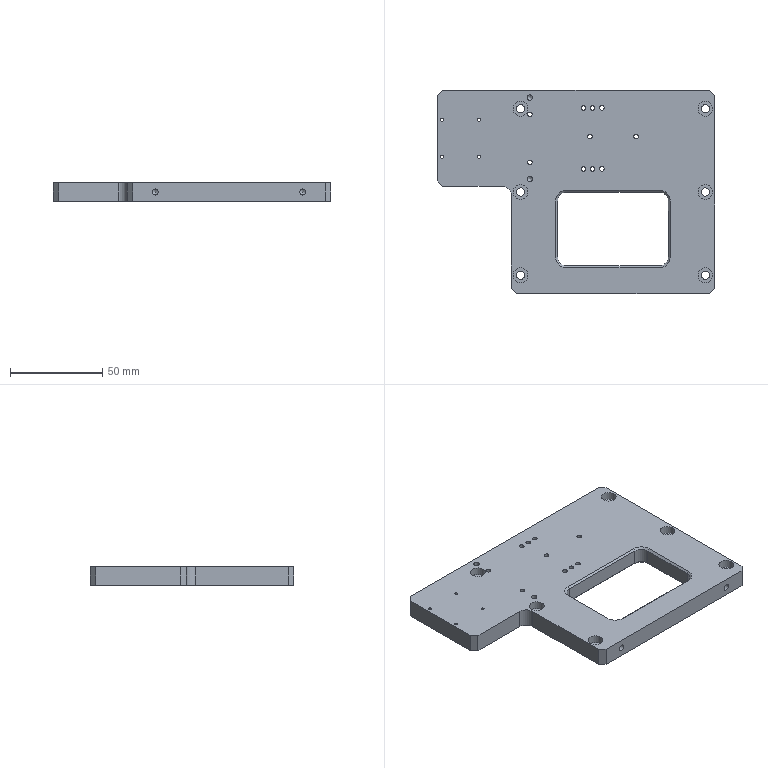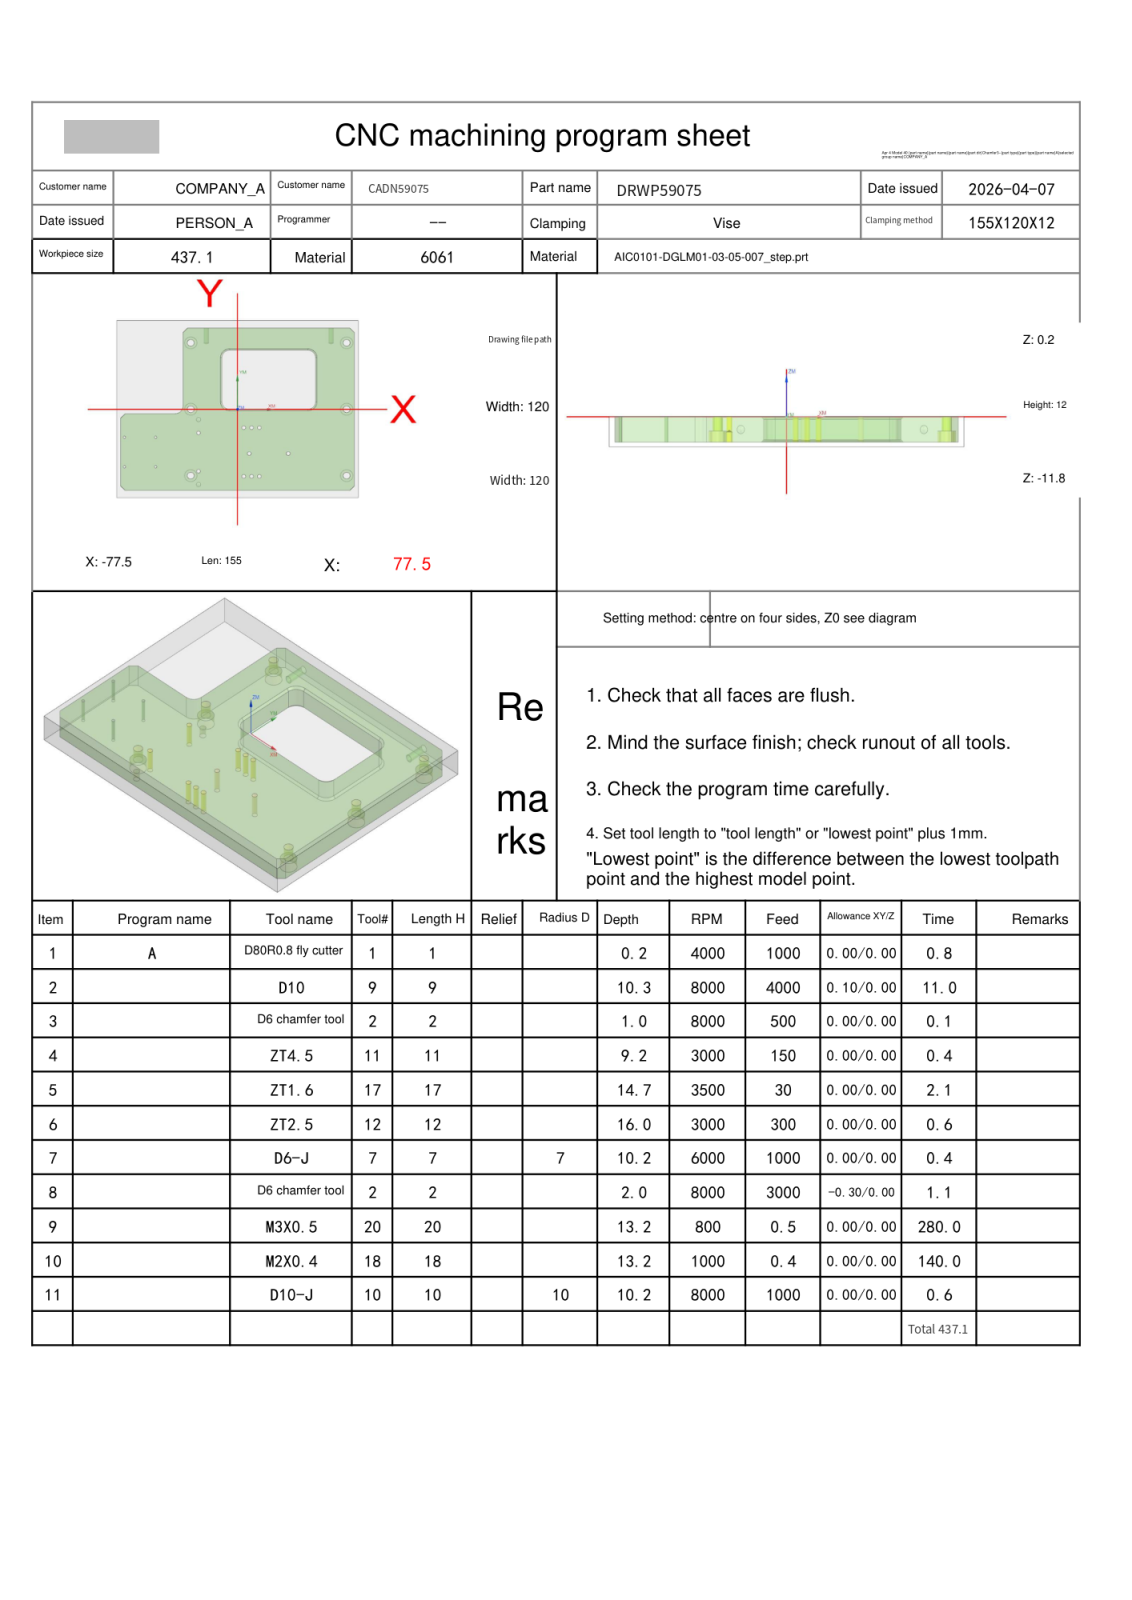NC program | NX | posted by the shop | part box 150 x 110 x 10 mm
Lines 41 to 1212 of 3675:
N2 T09 M06
(D10  D=10. R=0. H=09 ce=0.10 di=0.10)
G00 G90 G54 X-89.5 Y21.5 M03 S8000
G43 H09 Z10.2
M08
Z.719
G01 Z-.481 F4000.
X-85.
G03 X-78. Y28.5 I0.0 J7.
G01 Y60.
G02 X-77.5 Y60.5 I.5 J0.0
G01 X-35.464
G02 X-32. Y61.5 I3.464 J-5.5
G01 X72.
G02 X75.464 Y60.5 I0.0 J-6.5
G01 X77.5
G02 X78. Y60. I0.0 J-.5
G01 Y58.192
X79.596 Y56.596
G02 X81.5 Y52. I-4.596 J-4.596
G01 Y-52.
G02 X79.596 Y-56.596 I-6.5 J0.0
G01 X78. Y-58.192
Y-60.
G02 X77.5 Y-60.5 I-.5 J0.0
G01 X75.464
G02 X72. Y-61.5 I-3.464 J5.5
G01 X-72.
G02 X-75.464 Y-60.5 I0.0 J6.5
G01 X-77.5
G02 X-78. Y-60. I0.0 J.5
G01 Y-58.192
X-79.596 Y-56.596
G02 X-81.5 Y-52. I4.596 J4.596
G01 Y-6.
G02 X-79.596 Y-1.404 I6.5 J0.0
G01 X-78. Y.192
Y30.486
G02 X-77.582 Y31.299 I1. J0.0
G01 X-71.418 Y35.701
G03 X-71. Y36.514 I-.582 J.814
G01 Y52.503
G02 X-70.003 Y53.5 I1. J-.003
G01 X-42.48
G02 X-41.483 Y52.5 I-.003 J-1.
G01 X-41.485 Y52.436
G03 X-41.5 Y52. I6.485 J-.436
G01 Y4.497
G02 X-42.497 Y3.5 I-1. J.003
G01 X-69.511
G03 X-70.214 Y3.055 I0.0 J-.779
G01 X-70.383 Y2.7
X-70.423 Y2.52
G03 X-70.003 Y2.1 I.42 J0.0
G01 X-40.1
Y52.
G02 X-38.606 Y55.606 I5.1 J0.0
G01 X-35.606 Y58.606
G02 X-32. Y60.1 I3.606 J-3.606
G01 X72.
G02 X75.606 Y58.606 I0.0 J-5.1
G01 X78.606 Y55.606
G02 X80.1 Y52. I-3.606 J-3.606
G01 Y-52.
G02 X78.606 Y-55.606 I-5.1 J0.0
G01 X75.606 Y-58.606
G02 X72. Y-60.1 I-3.606 J3.606
G01 X-72.
G02 X-75.606 Y-58.606 I0.0 J5.1
G01 X-78.606 Y-55.606
G02 X-80.1 Y-52. I3.606 J3.606
G01 Y-6.
G02 X-78.606 Y-2.394 I5.1 J0.0
G01 X-75.606 Y.606
G02 X-72. Y2.1 I3.606 J-3.606
G01 X-70.003
G03 X-69.583 Y2.52 I0.0 J.42
G01 X-69.624 Y2.7
X-69.907 Y3.298
G03 X-70.191 Y3.518 I-.361 J-.172
G02 X-71. Y4.497 I.191 J.981
G01 Y30.486
G02 X-70.582 Y31.299 I1. J0.0
G01 X-64.418 Y35.701
G03 X-64. Y36.514 I-.582 J.814
G01 Y45.503
G02 X-63.003 Y46.5 I1. J-.003
G01 X-49.497
G02 X-48.5 Y45.503 I-.003 J-1.
G01 Y11.497
G02 X-49.497 Y10.5 I-1. J.003
G01 X-63.003
G02 X-64. Y11.497 I.003 J1.
G01 Y30.486
G02 X-63.582 Y31.299 I1. J0.0
G01 X-57.419 Y35.701
G03 X-57. Y36.514 I-.581 J.814
G01 Y38.803
G02 X-56.303 Y39.5 I.7 J-.003
G01 X-56.197
G02 X-55.5 Y38.803 I-.003 J-.7
G01 Y18.197
G02 X-56.197 Y17.5 I-.7 J.003
G01 X-56.303
G02 X-57. Y18.197 I.003 J.7
G01 Y33.5
Y34.
G03 X-64. Y41. I-7. J0.0
G01 X-89.5
Z.719
G00 Z3.
G01 Y21.5 F6000.
G00 Z.238
G01 Z-.962 F4000.
X-85.
G03 X-78. Y28.5 I0.0 J7.
G01 Y60.
G02 X-77.5 Y60.5 I.5 J0.0
G01 X-35.464
G02 X-32. Y61.5 I3.464 J-5.5
G01 X72.
G02 X75.464 Y60.5 I0.0 J-6.5
G01 X77.5
G02 X78. Y60. I0.0 J-.5
G01 Y58.192
X79.596 Y56.596
G02 X81.5 Y52. I-4.596 J-4.596
G01 Y-52.
G02 X79.596 Y-56.596 I-6.5 J0.0
G01 X78. Y-58.192
Y-60.
G02 X77.5 Y-60.5 I-.5 J0.0
G01 X75.464
G02 X72. Y-61.5 I-3.464 J5.5
G01 X-72.
G02 X-75.464 Y-60.5 I0.0 J6.5
G01 X-77.5
G02 X-78. Y-60. I0.0 J.5
G01 Y-58.192
X-79.596 Y-56.596
G02 X-81.5 Y-52. I4.596 J4.596
G01 Y-6.
G02 X-79.596 Y-1.404 I6.5 J0.0
G01 X-78. Y.192
Y33.5
G02 X-77.238 Y34.471 I1. J0.0
G01 X-71.762 Y35.813
G03 X-71. Y36.784 I-.238 J.971
G01 Y52.503
G02 X-70.003 Y53.5 I1. J-.003
G01 X-42.481
G02 X-41.483 Y52.5 I-.003 J-1.
G01 X-41.485 Y52.436
G03 X-41.5 Y52. I6.485 J-.436
G01 Y4.497
G02 X-42.497 Y3.5 I-1. J.003
G01 X-69.51
G03 X-70.214 Y3.055 I0.0 J-.779
G01 X-70.382 Y2.7
X-70.423 Y2.52
G03 X-70.003 Y2.1 I.42 J0.0
G01 X-40.1
Y52.
G02 X-38.606 Y55.606 I5.1 J0.0
G01 X-35.606 Y58.606
G02 X-32. Y60.1 I3.606 J-3.606
G01 X72.
G02 X75.606 Y58.606 I0.0 J-5.1
G01 X78.606 Y55.606
G02 X80.1 Y52. I-3.606 J-3.606
G01 Y-52.
G02 X78.606 Y-55.606 I-5.1 J0.0
G01 X75.606 Y-58.606
G02 X72. Y-60.1 I-3.606 J3.606
G01 X-72.
G02 X-75.606 Y-58.606 I0.0 J5.1
G01 X-78.606 Y-55.606
G02 X-80.1 Y-52. I3.606 J3.606
G01 Y-6.
G02 X-78.606 Y-2.394 I5.1 J0.0
G01 X-75.606 Y.606
G02 X-72. Y2.1 I3.606 J-3.606
G01 X-70.003
G03 X-69.583 Y2.52 I0.0 J.42
G01 X-69.623 Y2.7
X-69.906 Y3.298
G03 X-70.191 Y3.518 I-.361 J-.172
G02 X-71. Y4.497 I.191 J.982
G01 Y30.486
G02 X-70.582 Y31.299 I1. J0.0
G01 X-64.418 Y35.701
G03 X-64. Y36.514 I-.582 J.814
G01 Y45.503
G02 X-63.003 Y46.5 I1. J-.003
G01 X-49.497
G02 X-48.5 Y45.503 I-.003 J-1.
G01 Y11.497
G02 X-49.497 Y10.5 I-1. J.003
G01 X-63.003
G02 X-64. Y11.497 I.003 J1.
G01 Y30.486
G02 X-63.582 Y31.299 I1. J0.0
G01 X-57.419 Y35.701
G03 X-57. Y36.514 I-.581 J.814
G01 Y38.803
G02 X-56.303 Y39.5 I.7 J-.003
G01 X-56.197
G02 X-55.5 Y38.803 I-.003 J-.7
G01 Y18.197
G02 X-56.197 Y17.5 I-.7 J.003
G01 X-56.303
G02 X-57. Y18.197 I.003 J.7
G01 Y33.5
Y34.
G03 X-64. Y41. I-7. J0.0
G01 X-89.5
Z.238
G00 Z2.519
G01 Y21.5 F6000.
G00 Z-.243
G01 Z-1.443 F4000.
X-85.
G03 X-78. Y28.5 I0.0 J7.
G01 Y60.
G02 X-77.5 Y60.5 I.5 J0.0
G01 X-35.464
G02 X-32. Y61.5 I3.464 J-5.5
G01 X72.
G02 X75.464 Y60.5 I0.0 J-6.5
G01 X77.5
G02 X78. Y60. I0.0 J-.5
G01 Y58.192
X79.596 Y56.596
G02 X81.5 Y52. I-4.596 J-4.596
G01 Y-52.
G02 X79.596 Y-56.596 I-6.5 J0.0
G01 X78. Y-58.192
Y-60.
G02 X77.5 Y-60.5 I-.5 J0.0
G01 X75.464
G02 X72. Y-61.5 I-3.464 J5.5
G01 X-72.
G02 X-75.464 Y-60.5 I0.0 J6.5
G01 X-77.5
G02 X-78. Y-60. I0.0 J.5
G01 Y-58.192
X-79.596 Y-56.596
G02 X-81.5 Y-52. I4.596 J4.596
G01 Y-6.
G02 X-79.596 Y-1.404 I6.5 J0.0
G01 X-78. Y.192
Y33.5
G02 X-77.238 Y34.471 I1. J0.0
G01 X-71.762 Y35.813
G03 X-71. Y36.784 I-.238 J.971
G01 Y52.503
G02 X-70.003 Y53.5 I1. J-.003
G01 X-42.481
G02 X-41.483 Y52.5 I-.003 J-1.
G01 X-41.485 Y52.436
G03 X-41.5 Y52. I6.485 J-.436
G01 Y4.497
G02 X-42.497 Y3.5 I-1. J.003
G01 X-69.51
G03 X-70.214 Y3.055 I0.0 J-.779
G01 X-70.382 Y2.7
X-70.423 Y2.52
G03 X-70.003 Y2.1 I.42 J0.0
G01 X-40.1
Y52.
G02 X-38.606 Y55.606 I5.1 J0.0
G01 X-35.606 Y58.606
G02 X-32. Y60.1 I3.606 J-3.606
G01 X72.
G02 X75.606 Y58.606 I0.0 J-5.1
G01 X78.606 Y55.606
G02 X80.1 Y52. I-3.606 J-3.606
G01 Y-52.
G02 X78.606 Y-55.606 I-5.1 J0.0
G01 X75.606 Y-58.606
G02 X72. Y-60.1 I-3.606 J3.606
G01 X-72.
G02 X-75.606 Y-58.606 I0.0 J5.1
G01 X-78.606 Y-55.606
G02 X-80.1 Y-52. I3.606 J3.606
G01 Y-6.
G02 X-78.606 Y-2.394 I5.1 J0.0
G01 X-75.606 Y.606
G02 X-72. Y2.1 I3.606 J-3.606
G01 X-70.003
G03 X-69.583 Y2.52 I0.0 J.42
G01 X-69.623 Y2.7
X-69.906 Y3.298
G03 X-70.191 Y3.518 I-.361 J-.172
G02 X-71. Y4.497 I.191 J.982
G01 Y30.486
G02 X-70.582 Y31.299 I1. J0.0
G01 X-64.418 Y35.701
G03 X-64. Y36.514 I-.582 J.814
G01 Y45.503
G02 X-63.003 Y46.5 I1. J-.003
G01 X-49.497
G02 X-48.5 Y45.503 I-.003 J-1.
G01 Y11.497
G02 X-49.497 Y10.5 I-1. J.003
G01 X-63.003
G02 X-64. Y11.497 I.003 J1.
G01 Y30.486
G02 X-63.582 Y31.299 I1. J0.0
G01 X-57.419 Y35.701
G03 X-57. Y36.514 I-.581 J.814
G01 Y38.803
G02 X-56.303 Y39.5 I.7 J-.003
G01 X-56.197
G02 X-55.5 Y38.803 I-.003 J-.7
G01 Y18.197
G02 X-56.197 Y17.5 I-.7 J.003
G01 X-56.303
G02 X-57. Y18.197 I.003 J.7
G01 Y33.5
Y34.
G03 X-64. Y41. I-7. J0.0
G01 X-89.5
Z-.243
G00 Z2.038
G01 Y21.5 F6000.
G00 Z-.724
G01 Z-1.924 F4000.
X-85.
G03 X-78. Y28.5 I0.0 J7.
G01 Y60.
G02 X-77.5 Y60.5 I.5 J0.0
G01 X-35.464
G02 X-32. Y61.5 I3.464 J-5.5
G01 X72.
G02 X75.464 Y60.5 I0.0 J-6.5
G01 X77.5
G02 X78. Y60. I0.0 J-.5
G01 Y58.192
X79.596 Y56.596
G02 X81.5 Y52. I-4.596 J-4.596
G01 Y-52.
G02 X79.596 Y-56.596 I-6.5 J0.0
G01 X78. Y-58.192
Y-60.
G02 X77.5 Y-60.5 I-.5 J0.0
G01 X75.464
G02 X72. Y-61.5 I-3.464 J5.5
G01 X-72.
G02 X-75.464 Y-60.5 I0.0 J6.5
G01 X-77.5
G02 X-78. Y-60. I0.0 J.5
G01 Y-58.192
X-79.596 Y-56.596
G02 X-81.5 Y-52. I4.596 J4.596
G01 Y-6.
G02 X-79.596 Y-1.404 I6.5 J0.0
G01 X-78. Y.192
Y33.5
G02 X-77.238 Y34.471 I1. J0.0
G01 X-71.762 Y35.813
G03 X-71. Y36.784 I-.238 J.971
G01 Y52.503
G02 X-70.003 Y53.5 I1. J-.003
G01 X-42.481
G02 X-41.483 Y52.5 I-.003 J-1.
G01 X-41.485 Y52.436
G03 X-41.5 Y52. I6.485 J-.436
G01 Y4.497
G02 X-42.497 Y3.5 I-1. J.003
G01 X-69.51
G03 X-70.214 Y3.055 I0.0 J-.779
G01 X-70.382 Y2.7
X-70.423 Y2.52
G03 X-70.003 Y2.1 I.42 J0.0
G01 X-40.1
Y52.
G02 X-38.606 Y55.606 I5.1 J0.0
G01 X-35.606 Y58.606
G02 X-32. Y60.1 I3.606 J-3.606
G01 X72.
G02 X75.606 Y58.606 I0.0 J-5.1
G01 X78.606 Y55.606
G02 X80.1 Y52. I-3.606 J-3.606
G01 Y-52.
G02 X78.606 Y-55.606 I-5.1 J0.0
G01 X75.606 Y-58.606
G02 X72. Y-60.1 I-3.606 J3.606
G01 X-72.
G02 X-75.606 Y-58.606 I0.0 J5.1
G01 X-78.606 Y-55.606
G02 X-80.1 Y-52. I3.606 J3.606
G01 Y-6.
G02 X-78.606 Y-2.394 I5.1 J0.0
G01 X-75.606 Y.606
G02 X-72. Y2.1 I3.606 J-3.606
G01 X-70.003
G03 X-69.583 Y2.52 I0.0 J.42
G01 X-69.623 Y2.7
X-69.906 Y3.298
G03 X-70.191 Y3.518 I-.361 J-.172
G02 X-71. Y4.497 I.191 J.982
G01 Y30.486
G02 X-70.582 Y31.299 I1. J0.0
G01 X-64.418 Y35.701
G03 X-64. Y36.514 I-.582 J.814
G01 Y45.503
G02 X-63.003 Y46.5 I1. J-.003
G01 X-49.497
G02 X-48.5 Y45.503 I-.003 J-1.
G01 Y11.497
G02 X-49.497 Y10.5 I-1. J.003
G01 X-63.003
G02 X-64. Y11.497 I.003 J1.
G01 Y30.486
G02 X-63.582 Y31.299 I1. J0.0
G01 X-57.419 Y35.701
G03 X-57. Y36.514 I-.581 J.814
G01 Y38.803
G02 X-56.303 Y39.5 I.7 J-.003
G01 X-56.197
G02 X-55.5 Y38.803 I-.003 J-.7
G01 Y18.197
G02 X-56.197 Y17.5 I-.7 J.003
G01 X-56.303
G02 X-57. Y18.197 I.003 J.7
G01 Y33.5
Y34.
G03 X-64. Y41. I-7. J0.0
G01 X-89.5
Z-.724
G00 Z1.557
G01 Y21.5 F6000.
G00 Z-1.205
G01 Z-2.405 F4000.
X-85.
G03 X-78. Y28.5 I0.0 J7.
G01 Y60.
G02 X-77.5 Y60.5 I.5 J0.0
G01 X-35.464
G02 X-32. Y61.5 I3.464 J-5.5
G01 X72.
G02 X75.464 Y60.5 I0.0 J-6.5
G01 X77.5
G02 X78. Y60. I0.0 J-.5
G01 Y58.192
X79.596 Y56.596
G02 X81.5 Y52. I-4.596 J-4.596
G01 Y-52.
G02 X79.596 Y-56.596 I-6.5 J0.0
G01 X78. Y-58.192
Y-60.
G02 X77.5 Y-60.5 I-.5 J0.0
G01 X75.464
G02 X72. Y-61.5 I-3.464 J5.5
G01 X-72.
G02 X-75.464 Y-60.5 I0.0 J6.5
G01 X-77.5
G02 X-78. Y-60. I0.0 J.5
G01 Y-58.192
X-79.596 Y-56.596
G02 X-81.5 Y-52. I4.596 J4.596
G01 Y-6.
G02 X-79.596 Y-1.404 I6.5 J0.0
G01 X-78. Y.192
Y33.5
G02 X-77.238 Y34.471 I1. J0.0
G01 X-71.762 Y35.813
G03 X-71. Y36.784 I-.238 J.971
G01 Y52.503
G02 X-70.003 Y53.5 I1. J-.003
G01 X-42.481
G02 X-41.483 Y52.5 I-.003 J-1.
G01 X-41.485 Y52.436
G03 X-41.5 Y52. I6.485 J-.436
G01 Y4.497
G02 X-42.497 Y3.5 I-1. J.003
G01 X-69.51
G03 X-70.214 Y3.055 I0.0 J-.779
G01 X-70.382 Y2.7
X-70.423 Y2.52
G03 X-70.003 Y2.1 I.42 J0.0
G01 X-40.1
Y52.
G02 X-38.606 Y55.606 I5.1 J0.0
G01 X-35.606 Y58.606
G02 X-32. Y60.1 I3.606 J-3.606
G01 X72.
G02 X75.606 Y58.606 I0.0 J-5.1
G01 X78.606 Y55.606
G02 X80.1 Y52. I-3.606 J-3.606
G01 Y-52.
G02 X78.606 Y-55.606 I-5.1 J0.0
G01 X75.606 Y-58.606
G02 X72. Y-60.1 I-3.606 J3.606
G01 X-72.
G02 X-75.606 Y-58.606 I0.0 J5.1
G01 X-78.606 Y-55.606
G02 X-80.1 Y-52. I3.606 J3.606
G01 Y-6.
G02 X-78.606 Y-2.394 I5.1 J0.0
G01 X-75.606 Y.606
G02 X-72. Y2.1 I3.606 J-3.606
G01 X-70.003
G03 X-69.583 Y2.52 I0.0 J.42
G01 X-69.623 Y2.7
X-69.906 Y3.298
G03 X-70.191 Y3.518 I-.361 J-.172
G02 X-71. Y4.497 I.191 J.982
G01 Y30.486
G02 X-70.582 Y31.299 I1. J0.0
G01 X-64.418 Y35.701
G03 X-64. Y36.514 I-.582 J.814
G01 Y45.503
G02 X-63.003 Y46.5 I1. J-.003
G01 X-49.497
G02 X-48.5 Y45.503 I-.003 J-1.
G01 Y11.497
G02 X-49.497 Y10.5 I-1. J.003
G01 X-63.003
G02 X-64. Y11.497 I.003 J1.
G01 Y30.486
G02 X-63.582 Y31.299 I1. J0.0
G01 X-57.419 Y35.701
G03 X-57. Y36.514 I-.581 J.814
G01 Y38.803
G02 X-56.303 Y39.5 I.7 J-.003
G01 X-56.197
G02 X-55.5 Y38.803 I-.003 J-.7
G01 Y18.197
G02 X-56.197 Y17.5 I-.7 J.003
G01 X-56.303
G02 X-57. Y18.197 I.003 J.7
G01 Y33.5
Y34.
G03 X-64. Y41. I-7. J0.0
G01 X-89.5
Z-1.205
G00 Z1.076
G01 Y21.5 F6000.
G00 Z-1.686
G01 Z-2.886 F4000.
X-85.
G03 X-78. Y28.5 I0.0 J7.
G01 Y60.
G02 X-77.5 Y60.5 I.5 J0.0
G01 X-35.464
G02 X-32. Y61.5 I3.464 J-5.5
G01 X72.
G02 X75.464 Y60.5 I0.0 J-6.5
G01 X77.5
G02 X78. Y60. I0.0 J-.5
G01 Y58.192
X79.596 Y56.596
G02 X81.5 Y52. I-4.596 J-4.596
G01 Y-52.
G02 X79.596 Y-56.596 I-6.5 J0.0
G01 X78. Y-58.192
Y-60.
G02 X77.5 Y-60.5 I-.5 J0.0
G01 X75.464
G02 X72. Y-61.5 I-3.464 J5.5
G01 X-72.
G02 X-75.464 Y-60.5 I0.0 J6.5
G01 X-77.5
G02 X-78. Y-60. I0.0 J.5
G01 Y-58.192
X-79.596 Y-56.596
G02 X-81.5 Y-52. I4.596 J4.596
G01 Y-6.
G02 X-79.596 Y-1.404 I6.5 J0.0
G01 X-78. Y.192
Y33.5
G02 X-77.238 Y34.471 I1. J0.0
G01 X-71.762 Y35.813
G03 X-71. Y36.784 I-.238 J.971
G01 Y52.503
G02 X-70.003 Y53.5 I1. J-.003
G01 X-42.481
G02 X-41.483 Y52.5 I-.003 J-1.
G01 X-41.485 Y52.436
G03 X-41.5 Y52. I6.485 J-.436
G01 Y4.497
G02 X-42.497 Y3.5 I-1. J.003
G01 X-69.51
G03 X-70.214 Y3.055 I0.0 J-.779
G01 X-70.382 Y2.7
X-70.423 Y2.52
G03 X-70.003 Y2.1 I.42 J0.0
G01 X-40.1
Y52.
G02 X-38.606 Y55.606 I5.1 J0.0
G01 X-35.606 Y58.606
G02 X-32. Y60.1 I3.606 J-3.606
G01 X72.
G02 X75.606 Y58.606 I0.0 J-5.1
G01 X78.606 Y55.606
G02 X80.1 Y52. I-3.606 J-3.606
G01 Y-52.
G02 X78.606 Y-55.606 I-5.1 J0.0
G01 X75.606 Y-58.606
G02 X72. Y-60.1 I-3.606 J3.606
G01 X-72.
G02 X-75.606 Y-58.606 I0.0 J5.1
G01 X-78.606 Y-55.606
G02 X-80.1 Y-52. I3.606 J3.606
G01 Y-6.
G02 X-78.606 Y-2.394 I5.1 J0.0
G01 X-75.606 Y.606
G02 X-72. Y2.1 I3.606 J-3.606
G01 X-70.003
G03 X-69.583 Y2.52 I0.0 J.42
G01 X-69.623 Y2.7
X-69.906 Y3.298
G03 X-70.191 Y3.518 I-.361 J-.172
G02 X-71. Y4.497 I.191 J.982
G01 Y30.486
G02 X-70.582 Y31.299 I1. J0.0
G01 X-64.418 Y35.701
G03 X-64. Y36.514 I-.582 J.814
G01 Y45.503
G02 X-63.003 Y46.5 I1. J-.003
G01 X-49.497
G02 X-48.5 Y45.503 I-.003 J-1.
G01 Y11.497
G02 X-49.497 Y10.5 I-1. J.003
G01 X-63.003
G02 X-64. Y11.497 I.003 J1.
G01 Y30.486
G02 X-63.582 Y31.299 I1. J0.0
G01 X-57.419 Y35.701
G03 X-57. Y36.514 I-.581 J.814
G01 Y38.803
G02 X-56.303 Y39.5 I.7 J-.003
G01 X-56.197
G02 X-55.5 Y38.803 I-.003 J-.7
G01 Y18.197
G02 X-56.197 Y17.5 I-.7 J.003
G01 X-56.303
G02 X-57. Y18.197 I.003 J.7
G01 Y33.5
Y34.
G03 X-64. Y41. I-7. J0.0
G01 X-89.5
Z-1.686
G00 Z.595
G01 Y21.5 F6000.
G00 Z-2.167
G01 Z-3.367 F4000.
X-85.
G03 X-78. Y28.5 I0.0 J7.
G01 Y60.
G02 X-77.5 Y60.5 I.5 J0.0
G01 X-35.464
G02 X-32. Y61.5 I3.464 J-5.5
G01 X72.
G02 X75.464 Y60.5 I0.0 J-6.5
G01 X77.5
G02 X78. Y60. I0.0 J-.5
G01 Y58.192
X79.596 Y56.596
G02 X81.5 Y52. I-4.596 J-4.596
G01 Y-52.
G02 X79.596 Y-56.596 I-6.5 J0.0
G01 X78. Y-58.192
Y-60.
G02 X77.5 Y-60.5 I-.5 J0.0
G01 X75.464
G02 X72. Y-61.5 I-3.464 J5.5
G01 X-72.
G02 X-75.464 Y-60.5 I0.0 J6.5
G01 X-77.5
G02 X-78. Y-60. I0.0 J.5
G01 Y-58.192
X-79.596 Y-56.596
G02 X-81.5 Y-52. I4.596 J4.596
G01 Y-6.
G02 X-79.596 Y-1.404 I6.5 J0.0
G01 X-78. Y.192
Y33.5
G02 X-77.238 Y34.471 I1. J0.0
G01 X-71.762 Y35.813
G03 X-71. Y36.784 I-.238 J.971
G01 Y52.503
G02 X-70.003 Y53.5 I1. J-.003
G01 X-42.481
G02 X-41.483 Y52.5 I-.003 J-1.
G01 X-41.485 Y52.436
G03 X-41.5 Y52. I6.485 J-.436
G01 Y4.497
G02 X-42.497 Y3.5 I-1. J.003
G01 X-69.51
G03 X-70.214 Y3.055 I0.0 J-.779
G01 X-70.382 Y2.7
X-70.423 Y2.52
G03 X-70.003 Y2.1 I.42 J0.0
G01 X-40.1
Y52.
G02 X-38.606 Y55.606 I5.1 J0.0
G01 X-35.606 Y58.606
G02 X-32. Y60.1 I3.606 J-3.606
G01 X72.
G02 X75.606 Y58.606 I0.0 J-5.1
G01 X78.606 Y55.606
G02 X80.1 Y52. I-3.606 J-3.606
G01 Y-52.
G02 X78.606 Y-55.606 I-5.1 J0.0
G01 X75.606 Y-58.606
G02 X72. Y-60.1 I-3.606 J3.606
G01 X-72.
G02 X-75.606 Y-58.606 I0.0 J5.1
G01 X-78.606 Y-55.606
G02 X-80.1 Y-52. I3.606 J3.606
G01 Y-6.
G02 X-78.606 Y-2.394 I5.1 J0.0
G01 X-75.606 Y.606
G02 X-72. Y2.1 I3.606 J-3.606
G01 X-70.003
G03 X-69.583 Y2.52 I0.0 J.42
G01 X-69.623 Y2.7
X-69.906 Y3.298
G03 X-70.191 Y3.518 I-.361 J-.172
G02 X-71. Y4.497 I.191 J.982
G01 Y30.486
G02 X-70.582 Y31.299 I1. J0.0
G01 X-64.418 Y35.701
G03 X-64. Y36.514 I-.582 J.814
G01 Y45.503
G02 X-63.003 Y46.5 I1. J-.003
G01 X-49.497
G02 X-48.5 Y45.503 I-.003 J-1.
G01 Y11.497
G02 X-49.497 Y10.5 I-1. J.003
G01 X-63.003
G02 X-64. Y11.497 I.003 J1.
G01 Y30.486
G02 X-63.582 Y31.299 I1. J0.0
G01 X-57.419 Y35.701
G03 X-57. Y36.514 I-.581 J.814
G01 Y38.803
G02 X-56.303 Y39.5 I.7 J-.003
G01 X-56.197
G02 X-55.5 Y38.803 I-.003 J-.7
G01 Y18.197
G02 X-56.197 Y17.5 I-.7 J.003
G01 X-56.303
G02 X-57. Y18.197 I.003 J.7
G01 Y33.5
Y34.
G03 X-64. Y41. I-7. J0.0
G01 X-89.5
Z-2.167
G00 Z.114
G01 Y21.5 F6000.
G00 Z-2.648
G01 Z-3.848 F4000.
X-85.
G03 X-78. Y28.5 I0.0 J7.
G01 Y60.
G02 X-77.5 Y60.5 I.5 J0.0
G01 X-35.464
G02 X-32. Y61.5 I3.464 J-5.5
G01 X72.
G02 X75.464 Y60.5 I0.0 J-6.5
G01 X77.5
G02 X78. Y60. I0.0 J-.5
G01 Y58.192
X79.596 Y56.596
G02 X81.5 Y52. I-4.596 J-4.596
G01 Y-52.
G02 X79.596 Y-56.596 I-6.5 J0.0
G01 X78. Y-58.192
Y-60.
G02 X77.5 Y-60.5 I-.5 J0.0
G01 X75.464
G02 X72. Y-61.5 I-3.464 J5.5
G01 X-72.
G02 X-75.464 Y-60.5 I0.0 J6.5
G01 X-77.5
G02 X-78. Y-60. I0.0 J.5
G01 Y-58.192
X-79.596 Y-56.596
G02 X-81.5 Y-52. I4.596 J4.596
G01 Y-6.
G02 X-79.596 Y-1.404 I6.5 J0.0
G01 X-78. Y.192
Y33.5
G02 X-77.238 Y34.471 I1. J0.0
G01 X-71.762 Y35.813
G03 X-71. Y36.784 I-.238 J.971
G01 Y52.503
G02 X-70.003 Y53.5 I1. J-.003
G01 X-42.481
G02 X-41.483 Y52.5 I-.003 J-1.
G01 X-41.485 Y52.436
G03 X-41.5 Y52. I6.485 J-.436
G01 Y4.497
G02 X-42.497 Y3.5 I-1. J.003
G01 X-69.51
G03 X-70.214 Y3.055 I0.0 J-.779
G01 X-70.382 Y2.7
X-70.423 Y2.52
G03 X-70.003 Y2.1 I.42 J0.0
G01 X-40.1
Y52.
G02 X-38.606 Y55.606 I5.1 J0.0
G01 X-35.606 Y58.606
G02 X-32. Y60.1 I3.606 J-3.606
G01 X72.
G02 X75.606 Y58.606 I0.0 J-5.1
G01 X78.606 Y55.606
G02 X80.1 Y52. I-3.606 J-3.606
G01 Y-52.
G02 X78.606 Y-55.606 I-5.1 J0.0
G01 X75.606 Y-58.606
G02 X72. Y-60.1 I-3.606 J3.606
G01 X-72.
G02 X-75.606 Y-58.606 I0.0 J5.1
G01 X-78.606 Y-55.606
G02 X-80.1 Y-52. I3.606 J3.606
G01 Y-6.
G02 X-78.606 Y-2.394 I5.1 J0.0
G01 X-75.606 Y.606
G02 X-72. Y2.1 I3.606 J-3.606
G01 X-70.003
G03 X-69.583 Y2.52 I0.0 J.42
G01 X-69.623 Y2.7
X-69.906 Y3.298
G03 X-70.191 Y3.518 I-.361 J-.172
G02 X-71. Y4.497 I.191 J.982
G01 Y30.486
G02 X-70.582 Y31.299 I1. J0.0
G01 X-64.418 Y35.701
G03 X-64. Y36.514 I-.582 J.814
G01 Y45.503
G02 X-63.003 Y46.5 I1. J-.003
G01 X-49.497
G02 X-48.5 Y45.503 I-.003 J-1.
G01 Y11.497
G02 X-49.497 Y10.5 I-1. J.003
G01 X-63.003
G02 X-64. Y11.497 I.003 J1.
G01 Y30.486
G02 X-63.582 Y31.299 I1. J0.0
G01 X-57.419 Y35.701
G03 X-57. Y36.514 I-.581 J.814
G01 Y38.803
G02 X-56.303 Y39.5 I.7 J-.003
G01 X-56.197
G02 X-55.5 Y38.803 I-.003 J-.7
G01 Y18.197
G02 X-56.197 Y17.5 I-.7 J.003
G01 X-56.303
G02 X-57. Y18.197 I.003 J.7
G01 Y33.5
Y34.
G03 X-64. Y41. I-7. J0.0
G01 X-89.5
Z-2.648
G00 Z-.367
G01 Y21.5 F6000.
G00 Z-3.129
G01 Z-4.329 F4000.
X-85.
G03 X-78. Y28.5 I0.0 J7.
G01 Y60.
G02 X-77.5 Y60.5 I.5 J0.0
G01 X-35.464
G02 X-32. Y61.5 I3.464 J-5.5
G01 X72.
G02 X75.464 Y60.5 I0.0 J-6.5
G01 X77.5
G02 X78. Y60. I0.0 J-.5
G01 Y58.192
X79.596 Y56.596
G02 X81.5 Y52. I-4.596 J-4.596
G01 Y-52.
G02 X79.596 Y-56.596 I-6.5 J0.0
G01 X78. Y-58.192
Y-60.
G02 X77.5 Y-60.5 I-.5 J0.0
G01 X75.464
G02 X72. Y-61.5 I-3.464 J5.5
G01 X-72.
G02 X-75.464 Y-60.5 I0.0 J6.5
G01 X-77.5
G02 X-78. Y-60. I0.0 J.5
G01 Y-58.192
X-79.596 Y-56.596
G02 X-81.5 Y-52. I4.596 J4.596
G01 Y-6.
G02 X-79.596 Y-1.404 I6.5 J0.0
G01 X-78. Y.192
Y33.5
G02 X-77.238 Y34.471 I1. J0.0
G01 X-71.762 Y35.813
G03 X-71. Y36.784 I-.238 J.971
G01 Y52.503
G02 X-70.003 Y53.5 I1. J-.003
G01 X-42.481
G02 X-41.483 Y52.5 I-.003 J-1.
G01 X-41.485 Y52.436
G03 X-41.5 Y52. I6.485 J-.436
G01 Y4.497
G02 X-42.497 Y3.5 I-1. J.003
G01 X-69.51
G03 X-70.214 Y3.055 I0.0 J-.779
G01 X-70.382 Y2.7
X-70.423 Y2.52
G03 X-70.003 Y2.1 I.42 J0.0
G01 X-40.1
Y52.
G02 X-38.606 Y55.606 I5.1 J0.0
G01 X-35.606 Y58.606
G02 X-32. Y60.1 I3.606 J-3.606
G01 X72.
G02 X75.606 Y58.606 I0.0 J-5.1
G01 X78.606 Y55.606
G02 X80.1 Y52. I-3.606 J-3.606
G01 Y-52.
G02 X78.606 Y-55.606 I-5.1 J0.0
G01 X75.606 Y-58.606
G02 X72. Y-60.1 I-3.606 J3.606
G01 X-72.
G02 X-75.606 Y-58.606 I0.0 J5.1
G01 X-78.606 Y-55.606
G02 X-80.1 Y-52. I3.606 J3.606
G01 Y-6.
G02 X-78.606 Y-2.394 I5.1 J0.0
G01 X-75.606 Y.606
G02 X-72. Y2.1 I3.606 J-3.606
G01 X-70.003
G03 X-69.583 Y2.52 I0.0 J.42
G01 X-69.623 Y2.7
X-69.906 Y3.298
G03 X-70.191 Y3.518 I-.361 J-.172
G02 X-71. Y4.497 I.191 J.982
G01 Y30.486
G02 X-70.582 Y31.299 I1. J0.0
G01 X-64.418 Y35.701
G03 X-64. Y36.514 I-.582 J.814
G01 Y45.503
G02 X-63.003 Y46.5 I1. J-.003
G01 X-49.497
G02 X-48.5 Y45.503 I-.003 J-1.
G01 Y11.497
G02 X-49.497 Y10.5 I-1. J.003
G01 X-63.003
G02 X-64. Y11.497 I.003 J1.
G01 Y30.486
G02 X-63.582 Y31.299 I1. J0.0
G01 X-57.419 Y35.701
G03 X-57. Y36.514 I-.581 J.814
G01 Y38.803
G02 X-56.303 Y39.5 I.7 J-.003
G01 X-56.197
G02 X-55.5 Y38.803 I-.003 J-.7
G01 Y18.197
G02 X-56.197 Y17.5 I-.7 J.003
G01 X-56.303
G02 X-57. Y18.197 I.003 J.7
G01 Y33.5
Y34.
G03 X-64. Y41. I-7. J0.0
G01 X-89.5
Z-3.129
G00 Z-.848
G01 Y21.5 F6000.
G00 Z-3.61
G01 Z-4.81 F4000.
X-85.
G03 X-78. Y28.5 I0.0 J7.
G01 Y60.
G02 X-77.5 Y60.5 I.5 J0.0
G01 X-35.464
G02 X-32. Y61.5 I3.464 J-5.5
G01 X72.
G02 X75.464 Y60.5 I0.0 J-6.5
G01 X77.5
G02 X78. Y60. I0.0 J-.5
G01 Y58.192
X79.596 Y56.596
G02 X81.5 Y52. I-4.596 J-4.596
G01 Y-52.
G02 X79.596 Y-56.596 I-6.5 J0.0
G01 X78. Y-58.192
Y-60.
G02 X77.5 Y-60.5 I-.5 J0.0
G01 X75.464
G02 X72. Y-61.5 I-3.464 J5.5
G01 X-72.
G02 X-75.464 Y-60.5 I0.0 J6.5
G01 X-77.5
G02 X-78. Y-60. I0.0 J.5
G01 Y-58.192
X-79.596 Y-56.596
G02 X-81.5 Y-52. I4.596 J4.596
G01 Y-6.
G02 X-79.596 Y-1.404 I6.5 J0.0
G01 X-78. Y.192
Y33.5
G02 X-77.238 Y34.471 I1. J0.0
G01 X-71.762 Y35.813
G03 X-71. Y36.784 I-.238 J.971
G01 Y52.503
G02 X-70.003 Y53.5 I1. J-.003
G01 X-42.481
G02 X-41.483 Y52.5 I-.003 J-1.
G01 X-41.485 Y52.436
G03 X-41.5 Y52. I6.485 J-.436
G01 Y4.497
G02 X-42.497 Y3.5 I-1. J.003
G01 X-69.51
G03 X-70.214 Y3.055 I0.0 J-.779
G01 X-70.382 Y2.7
X-70.423 Y2.52
G03 X-70.003 Y2.1 I.42 J0.0
G01 X-40.1
Y52.
G02 X-38.606 Y55.606 I5.1 J0.0
G01 X-35.606 Y58.606
G02 X-32. Y60.1 I3.606 J-3.606
G01 X72.
G02 X75.606 Y58.606 I0.0 J-5.1
G01 X78.606 Y55.606
G02 X80.1 Y52. I-3.606 J-3.606
G01 Y-52.
G02 X78.606 Y-55.606 I-5.1 J0.0
G01 X75.606 Y-58.606
G02 X72. Y-60.1 I-3.606 J3.606
G01 X-72.
G02 X-75.606 Y-58.606 I0.0 J5.1
G01 X-78.606 Y-55.606
G02 X-80.1 Y-52. I3.606 J3.606
G01 Y-6.
G02 X-78.606 Y-2.394 I5.1 J0.0
G01 X-75.606 Y.606
G02 X-72. Y2.1 I3.606 J-3.606
G01 X-70.003
G03 X-69.583 Y2.52 I0.0 J.42
G01 X-69.623 Y2.7
X-69.906 Y3.298
G03 X-70.191 Y3.518 I-.361 J-.172
G02 X-71. Y4.497 I.191 J.982
G01 Y30.486
G02 X-70.582 Y31.299 I1. J0.0
G01 X-64.418 Y35.701
G03 X-64. Y36.514 I-.582 J.814
G01 Y45.503
G02 X-63.003 Y46.5 I1. J-.003
G01 X-49.497
G02 X-48.5 Y45.503 I-.003 J-1.
G01 Y11.497
G02 X-49.497 Y10.5 I-1. J.003
G01 X-63.003
G02 X-64. Y11.497 I.003 J1.
G01 Y30.486
G02 X-63.582 Y31.299 I1. J0.0
G01 X-57.419 Y35.701
G03 X-57. Y36.514 I-.581 J.814
G01 Y38.803
G02 X-56.303 Y39.5 I.7 J-.003
G01 X-56.197
G02 X-55.5 Y38.803 I-.003 J-.7
G01 Y18.197
G02 X-56.197 Y17.5 I-.7 J.003
G01 X-56.303
G02 X-57. Y18.197 I.003 J.7
G01 Y33.5
Y34.
G03 X-64. Y41. I-7. J0.0
G01 X-89.5
Z-3.61
G00 Z-1.329
G01 Y21.5 F6000.
G00 Z-4.09
G01 Z-5.29 F4000.
X-85.
G03 X-78. Y28.5 I0.0 J7.
G01 Y60.
G02 X-77.5 Y60.5 I.5 J0.0
G01 X-35.464
G02 X-32. Y61.5 I3.464 J-5.5
G01 X72.
G02 X75.464 Y60.5 I0.0 J-6.5
G01 X77.5
G02 X78. Y60. I0.0 J-.5
G01 Y58.192
X79.596 Y56.596
G02 X81.5 Y52. I-4.596 J-4.596
G01 Y-52.
G02 X79.596 Y-56.596 I-6.5 J0.0
G01 X78. Y-58.192
Y-60.
G02 X77.5 Y-60.5 I-.5 J0.0
G01 X75.464
G02 X72. Y-61.5 I-3.464 J5.5
G01 X-72.
G02 X-75.464 Y-60.5 I0.0 J6.5
G01 X-77.5
G02 X-78. Y-60. I0.0 J.5
G01 Y-58.192
X-79.596 Y-56.596
G02 X-81.5 Y-52. I4.596 J4.596
G01 Y-6.
G02 X-79.596 Y-1.404 I6.5 J0.0
G01 X-78. Y.192
Y33.5
G02 X-77.238 Y34.471 I1. J0.0
G01 X-71.762 Y35.813
G03 X-71. Y36.784 I-.238 J.971
G01 Y52.503
G02 X-70.003 Y53.5 I1. J-.003
G01 X-42.481
G02 X-41.483 Y52.5 I-.003 J-1.
G01 X-41.485 Y52.436
G03 X-41.5 Y52. I6.485 J-.436
G01 Y4.497
G02 X-42.497 Y3.5 I-1. J.003
G01 X-69.51
G03 X-70.214 Y3.055 I0.0 J-.779
G01 X-70.382 Y2.7
X-70.423 Y2.52
G03 X-70.003 Y2.1 I.42 J0.0
G01 X-40.1
Y52.
G02 X-38.606 Y55.606 I5.1 J0.0
G01 X-35.606 Y58.606
G02 X-32. Y60.1 I3.606 J-3.606
G01 X72.
G02 X75.606 Y58.606 I0.0 J-5.1
G01 X78.606 Y55.606
G02 X80.1 Y52. I-3.606 J-3.606
G01 Y-52.
G02 X78.606 Y-55.606 I-5.1 J0.0
G01 X75.606 Y-58.606
G02 X72. Y-60.1 I-3.606 J3.606
G01 X-72.
G02 X-75.606 Y-58.606 I0.0 J5.1
G01 X-78.606 Y-55.606
G02 X-80.1 Y-52. I3.606 J3.606
G01 Y-6.
G02 X-78.606 Y-2.394 I5.1 J0.0
G01 X-75.606 Y.606
G02 X-72. Y2.1 I3.606 J-3.606
G01 X-70.003
G03 X-69.583 Y2.52 I0.0 J.42
G01 X-69.623 Y2.7
X-69.906 Y3.298
G03 X-70.191 Y3.518 I-.361 J-.172
G02 X-71. Y4.497 I.191 J.982
G01 Y30.486
G02 X-70.582 Y31.299 I1. J0.0
G01 X-64.418 Y35.701
G03 X-64. Y36.514 I-.582 J.814
G01 Y45.503
G02 X-63.003 Y46.5 I1. J-.003
G01 X-49.497
G02 X-48.5 Y45.503 I-.003 J-1.
G01 Y11.497
G02 X-49.497 Y10.5 I-1. J.003
G01 X-63.003
G02 X-64. Y11.497 I.003 J1.
G01 Y30.486
G02 X-63.582 Y31.299 I1. J0.0
G01 X-57.419 Y35.701
G03 X-57. Y36.514 I-.581 J.814
G01 Y38.803
G02 X-56.303 Y39.5 I.7 J-.003
G01 X-56.197
G02 X-55.5 Y38.803 I-.003 J-.7
G01 Y18.197